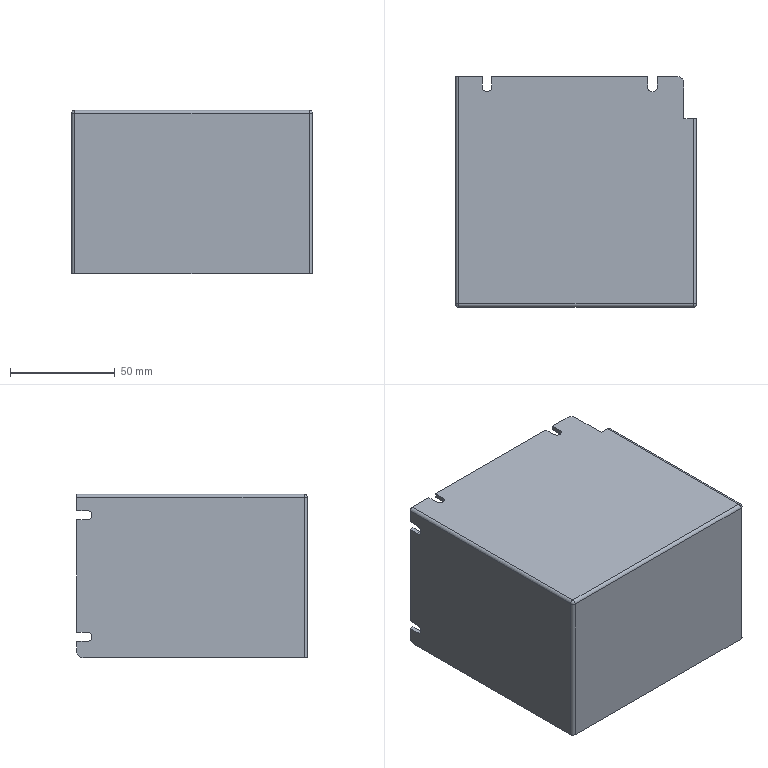Part | STEP file | 1 solid | 38 faces | box 115 x 110 x 78 mm | volume 71850 mm3 | plane 24 | cylinder 12 | sphere 2 | commonest cylinder face diameters 3 x5 4.5 x4 6 x3